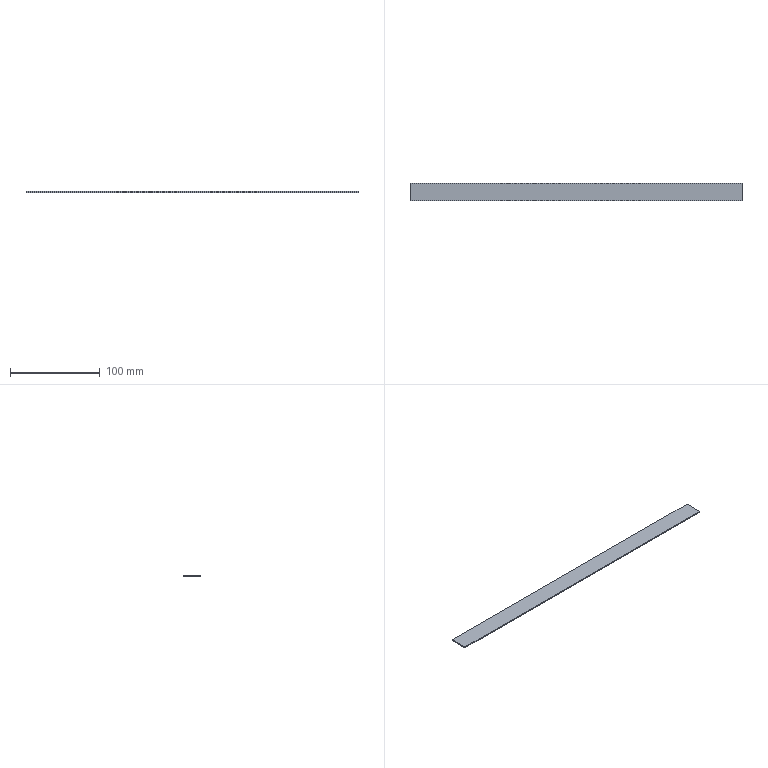Part | SolidWorks | features BaseBody 1 | 1 solid | 6 faces | box 370 x 20 x 1.2 mm | volume 8880 mm3 | plane 6
STEP:
#1=CARTESIAN_POINT('',(-185.,10.,0.));
#2=VERTEX_POINT('',#1);
#3=CARTESIAN_POINT('',(-185.,-10.,0.));
#4=VERTEX_POINT('',#3);
#5=CARTESIAN_POINT('',(-185.,10.,0.));
#6=DIRECTION('',(0.,-1.,0.));
#7=VECTOR('',#6,1000.);
#8=LINE('',#5,#7);
#9=EDGE_CURVE('',#2,#4,#8,.T.);
#10=ORIENTED_EDGE('',*,*,#9,.T.);
#11=CARTESIAN_POINT('',(185.,-10.,0.));
#12=VERTEX_POINT('',#11);
#13=CARTESIAN_POINT('',(185.,-10.,0.));
#14=DIRECTION('',(1.,0.,0.));
#15=VECTOR('',#14,1000.);
#16=LINE('',#13,#15);
#17=EDGE_CURVE('',#4,#12,#16,.T.);
#18=ORIENTED_EDGE('',*,*,#17,.T.);
#19=CARTESIAN_POINT('',(185.,10.,0.));
#20=VERTEX_POINT('',#19);
#21=CARTESIAN_POINT('',(185.,10.,0.));
#22=DIRECTION('',(0.,1.,0.));
#23=VECTOR('',#22,1000.);
#24=LINE('',#21,#23);
#25=EDGE_CURVE('',#12,#20,#24,.T.);
#26=ORIENTED_EDGE('',*,*,#25,.T.);
#27=CARTESIAN_POINT('',(185.,10.,0.));
#28=DIRECTION('',(-1.,0.,0.));
#29=VECTOR('',#28,1000.);
#30=LINE('',#27,#29);
#31=EDGE_CURVE('',#20,#2,#30,.T.);
#32=ORIENTED_EDGE('',*,*,#31,.T.);
#33=EDGE_LOOP('',(#10,#18,#26,#32));
#34=FACE_OUTER_BOUND('',#33,.T.);
#35=CARTESIAN_POINT('',(0.,0.,0.));
#36=DIRECTION('',(0.,0.,-1.));
#37=DIRECTION('',(0.,-1.,0.));
#38=AXIS2_PLACEMENT_3D('',#35,#36,#37);
#39=PLANE('',#38);
#40=ADVANCED_FACE('',(#34),#39,.F.);
#41=CARTESIAN_POINT('',(-185.,10.,-1.2));
#42=VERTEX_POINT('',#41);
#43=CARTESIAN_POINT('',(-185.,-10.,-1.2));
#44=VERTEX_POINT('',#43);
#45=CARTESIAN_POINT('',(-185.,10.,-1.2));
#46=DIRECTION('',(0.,-1.,0.));
#47=VECTOR('',#46,1000.);
#48=LINE('',#45,#47);
#49=EDGE_CURVE('',#42,#44,#48,.T.);
#50=ORIENTED_EDGE('',*,*,#49,.F.);
#51=CARTESIAN_POINT('',(185.,10.,-1.2));
#52=VERTEX_POINT('',#51);
#53=CARTESIAN_POINT('',(185.,10.,-1.2));
#54=DIRECTION('',(-1.,0.,0.));
#55=VECTOR('',#54,1000.);
#56=LINE('',#53,#55);
#57=EDGE_CURVE('',#52,#42,#56,.T.);
#58=ORIENTED_EDGE('',*,*,#57,.F.);
#59=CARTESIAN_POINT('',(185.,-10.,-1.2));
#60=VERTEX_POINT('',#59);
#61=CARTESIAN_POINT('',(185.,10.,-1.2));
#62=DIRECTION('',(0.,1.,0.));
#63=VECTOR('',#62,1000.);
#64=LINE('',#61,#63);
#65=EDGE_CURVE('',#60,#52,#64,.T.);
#66=ORIENTED_EDGE('',*,*,#65,.F.);
#67=CARTESIAN_POINT('',(185.,-10.,-1.2));
#68=DIRECTION('',(1.,0.,0.));
#69=VECTOR('',#68,1000.);
#70=LINE('',#67,#69);
#71=EDGE_CURVE('',#44,#60,#70,.T.);
#72=ORIENTED_EDGE('',*,*,#71,.F.);
#73=EDGE_LOOP('',(#50,#58,#66,#72));
#74=FACE_OUTER_BOUND('',#73,.T.);
#75=CARTESIAN_POINT('',(0.,0.,-1.2));
#76=DIRECTION('',(0.,0.,-1.));
#77=DIRECTION('',(0.,-1.,0.));
#78=AXIS2_PLACEMENT_3D('',#75,#76,#77);
#79=PLANE('',#78);
#80=ADVANCED_FACE('',(#74),#79,.T.);
#81=ORIENTED_EDGE('',*,*,#17,.F.);
#82=CARTESIAN_POINT('',(-185.,-10.,-1.2));
#83=DIRECTION('',(0.,0.,1.));
#84=VECTOR('',#83,1000.);
#85=LINE('',#82,#84);
#86=EDGE_CURVE('',#44,#4,#85,.T.);
#87=ORIENTED_EDGE('',*,*,#86,.F.);
#88=ORIENTED_EDGE('',*,*,#71,.T.);
#89=CARTESIAN_POINT('',(185.,-10.,-1.2));
#90=DIRECTION('',(0.,0.,1.));
#91=VECTOR('',#90,1000.);
#92=LINE('',#89,#91);
#93=EDGE_CURVE('',#60,#12,#92,.T.);
#94=ORIENTED_EDGE('',*,*,#93,.T.);
#95=EDGE_LOOP('',(#81,#87,#88,#94));
#96=FACE_OUTER_BOUND('',#95,.T.);
#97=CARTESIAN_POINT('',(185.,-10.,-1.2));
#98=DIRECTION('',(0.,-1.,0.));
#99=DIRECTION('',(0.,0.,-1.));
#100=AXIS2_PLACEMENT_3D('',#97,#98,#99);
#101=PLANE('',#100);
#102=ADVANCED_FACE('',(#96),#101,.T.);
#103=ORIENTED_EDGE('',*,*,#25,.F.);
#104=ORIENTED_EDGE('',*,*,#93,.F.);
#105=ORIENTED_EDGE('',*,*,#65,.T.);
#106=CARTESIAN_POINT('',(185.,10.,-1.2));
#107=DIRECTION('',(0.,0.,1.));
#108=VECTOR('',#107,1000.);
#109=LINE('',#106,#108);
#110=EDGE_CURVE('',#52,#20,#109,.T.);
#111=ORIENTED_EDGE('',*,*,#110,.T.);
#112=EDGE_LOOP('',(#103,#104,#105,#111));
#113=FACE_OUTER_BOUND('',#112,.T.);
#114=CARTESIAN_POINT('',(185.,10.,-1.2));
#115=DIRECTION('',(1.,0.,0.));
#116=DIRECTION('',(0.,1.,0.));
#117=AXIS2_PLACEMENT_3D('',#114,#115,#116);
#118=PLANE('',#117);
#119=ADVANCED_FACE('',(#113),#118,.T.);
#120=ORIENTED_EDGE('',*,*,#31,.F.);
#121=ORIENTED_EDGE('',*,*,#110,.F.);
#122=ORIENTED_EDGE('',*,*,#57,.T.);
#123=CARTESIAN_POINT('',(-185.,10.,-1.2));
#124=DIRECTION('',(0.,0.,1.));
#125=VECTOR('',#124,1000.);
#126=LINE('',#123,#125);
#127=EDGE_CURVE('',#42,#2,#126,.T.);
#128=ORIENTED_EDGE('',*,*,#127,.T.);
#129=EDGE_LOOP('',(#120,#121,#122,#128));
#130=FACE_OUTER_BOUND('',#129,.T.);
#131=CARTESIAN_POINT('',(185.,10.,-1.2));
#132=DIRECTION('',(0.,1.,0.));
#133=DIRECTION('',(1.,0.,0.));
#134=AXIS2_PLACEMENT_3D('',#131,#132,#133);
#135=PLANE('',#134);
#136=ADVANCED_FACE('',(#130),#135,.T.);
#137=ORIENTED_EDGE('',*,*,#9,.F.);
#138=ORIENTED_EDGE('',*,*,#127,.F.);
#139=ORIENTED_EDGE('',*,*,#49,.T.);
#140=ORIENTED_EDGE('',*,*,#86,.T.);
#141=EDGE_LOOP('',(#137,#138,#139,#140));
#142=FACE_OUTER_BOUND('',#141,.T.);
#143=CARTESIAN_POINT('',(-185.,10.,-1.2));
#144=DIRECTION('',(-1.,0.,0.));
#145=DIRECTION('',(0.,0.,1.));
#146=AXIS2_PLACEMENT_3D('',#143,#144,#145);
#147=PLANE('',#146);
#148=ADVANCED_FACE('',(#142),#147,.T.);
#149=CLOSED_SHELL('',(#40,#80,#102,#119,#136,#148));
#150=MANIFOLD_SOLID_BREP('',#149);
#151=CARTESIAN_POINT('',(0.,0.,0.));
#152=DIRECTION('',(0.,0.,1.));
#153=DIRECTION('',(1.,0.,0.));
#154=AXIS2_PLACEMENT_3D('',#151,#152,#153);
#155=(LENGTH_UNIT()NAMED_UNIT(*)SI_UNIT(.MILLI.,.METRE.));
#156=UNCERTAINTY_MEASURE_WITH_UNIT(LENGTH_MEASURE(0.00001),#155,'','');
#157=(NAMED_UNIT(*)PLANE_ANGLE_UNIT()SI_UNIT($,.RADIAN.));
#158=(NAMED_UNIT(*)SI_UNIT($,.STERADIAN.)SOLID_ANGLE_UNIT());
#159=(GEOMETRIC_REPRESENTATION_CONTEXT(3)GLOBAL_UNCERTAINTY_ASSIGNED_CONTEXT((#156))GLOBAL_UNIT_ASSIGNED_CONTEXT((#155,#157,#158))REPRESENTATION_CONTEXT('',''));
#160=ADVANCED_BREP_SHAPE_REPRESENTATION('',(#150,#154),#159);